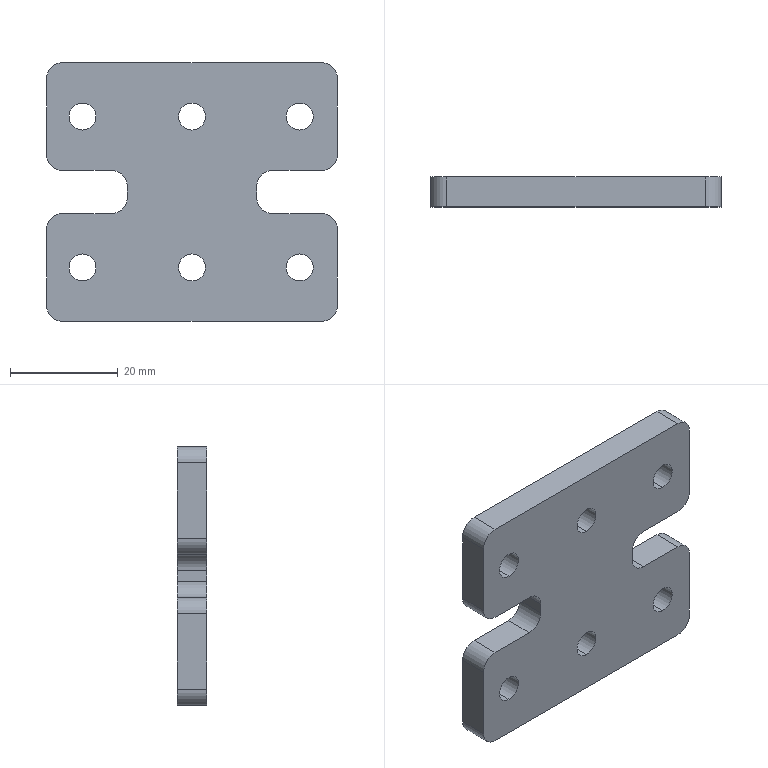Part | SolidWorks | features BaseBody 1 | 1 solid | 38 faces | box 54 x 5.5 x 48 mm | volume 12246 mm3 | cylinder 24 | plane 14 | commonest cylinder face diameters 5 x12 6 x12
STEP:
#1=CARTESIAN_POINT('',(20.,0.,11.5));
#2=VERTEX_POINT('',#1);
#3=CARTESIAN_POINT('',(20.,0.,16.5));
#4=VERTEX_POINT('',#3);
#5=CARTESIAN_POINT('',(20.,0.,14.));
#6=DIRECTION('',(0.,1.,0.));
#7=DIRECTION('',(0.,0.,1.));
#8=AXIS2_PLACEMENT_3D('',#5,#6,#7);
#9=CIRCLE('',#8,2.5);
#10=EDGE_CURVE('',#2,#4,#9,.T.);
#11=ORIENTED_EDGE('',*,*,#10,.F.);
#12=CARTESIAN_POINT('',(20.,5.5,11.5));
#13=VERTEX_POINT('',#12);
#14=CARTESIAN_POINT('',(20.,0.,11.5));
#15=DIRECTION('',(0.,1.,0.));
#16=VECTOR('',#15,1000.);
#17=LINE('',#14,#16);
#18=EDGE_CURVE('',#2,#13,#17,.T.);
#19=ORIENTED_EDGE('',*,*,#18,.T.);
#20=CARTESIAN_POINT('',(20.,5.5,16.5));
#21=VERTEX_POINT('',#20);
#22=CARTESIAN_POINT('',(20.,5.5,14.));
#23=DIRECTION('',(0.,-1.,0.));
#24=DIRECTION('',(0.,0.,1.));
#25=AXIS2_PLACEMENT_3D('',#22,#23,#24);
#26=CIRCLE('',#25,2.5);
#27=EDGE_CURVE('',#21,#13,#26,.T.);
#28=ORIENTED_EDGE('',*,*,#27,.F.);
#29=CARTESIAN_POINT('',(20.,0.,16.5));
#30=DIRECTION('',(0.,1.,0.));
#31=VECTOR('',#30,1000.);
#32=LINE('',#29,#31);
#33=EDGE_CURVE('',#4,#21,#32,.T.);
#34=ORIENTED_EDGE('',*,*,#33,.F.);
#35=EDGE_LOOP('',(#11,#19,#28,#34));
#36=FACE_OUTER_BOUND('',#35,.T.);
#37=CARTESIAN_POINT('',(20.,0.,14.));
#38=DIRECTION('',(0.,1.,0.));
#39=DIRECTION('',(0.,0.,1.));
#40=AXIS2_PLACEMENT_3D('',#37,#38,#39);
#41=CYLINDRICAL_SURFACE('',#40,2.5);
#42=ADVANCED_FACE('',(#36),#41,.F.);
#43=CARTESIAN_POINT('',(0.,0.,-16.5));
#44=VERTEX_POINT('',#43);
#45=CARTESIAN_POINT('',(0.,0.,-11.5));
#46=VERTEX_POINT('',#45);
#47=CARTESIAN_POINT('',(0.,0.,-14.));
#48=DIRECTION('',(0.,1.,0.));
#49=DIRECTION('',(0.,0.,1.));
#50=AXIS2_PLACEMENT_3D('',#47,#48,#49);
#51=CIRCLE('',#50,2.5);
#52=EDGE_CURVE('',#44,#46,#51,.T.);
#53=ORIENTED_EDGE('',*,*,#52,.F.);
#54=CARTESIAN_POINT('',(0.,5.5,-16.5));
#55=VERTEX_POINT('',#54);
#56=CARTESIAN_POINT('',(0.,0.,-16.5));
#57=DIRECTION('',(0.,1.,0.));
#58=VECTOR('',#57,1000.);
#59=LINE('',#56,#58);
#60=EDGE_CURVE('',#44,#55,#59,.T.);
#61=ORIENTED_EDGE('',*,*,#60,.T.);
#62=CARTESIAN_POINT('',(0.,5.5,-11.5));
#63=VERTEX_POINT('',#62);
#64=CARTESIAN_POINT('',(0.,5.5,-14.));
#65=DIRECTION('',(0.,-1.,0.));
#66=DIRECTION('',(0.,0.,1.));
#67=AXIS2_PLACEMENT_3D('',#64,#65,#66);
#68=CIRCLE('',#67,2.5);
#69=EDGE_CURVE('',#63,#55,#68,.T.);
#70=ORIENTED_EDGE('',*,*,#69,.F.);
#71=CARTESIAN_POINT('',(0.,0.,-11.5));
#72=DIRECTION('',(0.,1.,0.));
#73=VECTOR('',#72,1000.);
#74=LINE('',#71,#73);
#75=EDGE_CURVE('',#46,#63,#74,.T.);
#76=ORIENTED_EDGE('',*,*,#75,.F.);
#77=EDGE_LOOP('',(#53,#61,#70,#76));
#78=FACE_OUTER_BOUND('',#77,.T.);
#79=CARTESIAN_POINT('',(0.,0.,-14.));
#80=DIRECTION('',(0.,1.,0.));
#81=DIRECTION('',(0.,0.,1.));
#82=AXIS2_PLACEMENT_3D('',#79,#80,#81);
#83=CYLINDRICAL_SURFACE('',#82,2.5);
#84=ADVANCED_FACE('',(#78),#83,.F.);
#85=CARTESIAN_POINT('',(-20.32,0.,-16.5));
#86=VERTEX_POINT('',#85);
#87=CARTESIAN_POINT('',(-20.32,0.,-11.5));
#88=VERTEX_POINT('',#87);
#89=CARTESIAN_POINT('',(-20.32,0.,-14.));
#90=DIRECTION('',(0.,1.,0.));
#91=DIRECTION('',(0.,0.,1.));
#92=AXIS2_PLACEMENT_3D('',#89,#90,#91);
#93=CIRCLE('',#92,2.5);
#94=EDGE_CURVE('',#86,#88,#93,.T.);
#95=ORIENTED_EDGE('',*,*,#94,.F.);
#96=CARTESIAN_POINT('',(-20.32,5.5,-16.5));
#97=VERTEX_POINT('',#96);
#98=CARTESIAN_POINT('',(-20.32,0.,-16.5));
#99=DIRECTION('',(0.,1.,0.));
#100=VECTOR('',#99,1000.);
#101=LINE('',#98,#100);
#102=EDGE_CURVE('',#86,#97,#101,.T.);
#103=ORIENTED_EDGE('',*,*,#102,.T.);
#104=CARTESIAN_POINT('',(-20.32,5.5,-11.5));
#105=VERTEX_POINT('',#104);
#106=CARTESIAN_POINT('',(-20.32,5.5,-14.));
#107=DIRECTION('',(0.,-1.,0.));
#108=DIRECTION('',(0.,0.,1.));
#109=AXIS2_PLACEMENT_3D('',#106,#107,#108);
#110=CIRCLE('',#109,2.5);
#111=EDGE_CURVE('',#105,#97,#110,.T.);
#112=ORIENTED_EDGE('',*,*,#111,.F.);
#113=CARTESIAN_POINT('',(-20.32,0.,-11.5));
#114=DIRECTION('',(0.,1.,0.));
#115=VECTOR('',#114,1000.);
#116=LINE('',#113,#115);
#117=EDGE_CURVE('',#88,#105,#116,.T.);
#118=ORIENTED_EDGE('',*,*,#117,.F.);
#119=EDGE_LOOP('',(#95,#103,#112,#118));
#120=FACE_OUTER_BOUND('',#119,.T.);
#121=CARTESIAN_POINT('',(-20.32,0.,-14.));
#122=DIRECTION('',(0.,1.,0.));
#123=DIRECTION('',(0.,0.,1.));
#124=AXIS2_PLACEMENT_3D('',#121,#122,#123);
#125=CYLINDRICAL_SURFACE('',#124,2.5);
#126=ADVANCED_FACE('',(#120),#125,.F.);
#127=CARTESIAN_POINT('',(0.,0.,11.5));
#128=VERTEX_POINT('',#127);
#129=CARTESIAN_POINT('',(0.,0.,16.5));
#130=VERTEX_POINT('',#129);
#131=CARTESIAN_POINT('',(0.,0.,14.));
#132=DIRECTION('',(0.,1.,0.));
#133=DIRECTION('',(0.,0.,1.));
#134=AXIS2_PLACEMENT_3D('',#131,#132,#133);
#135=CIRCLE('',#134,2.5);
#136=EDGE_CURVE('',#128,#130,#135,.T.);
#137=ORIENTED_EDGE('',*,*,#136,.F.);
#138=CARTESIAN_POINT('',(0.,5.5,11.5));
#139=VERTEX_POINT('',#138);
#140=CARTESIAN_POINT('',(0.,0.,11.5));
#141=DIRECTION('',(0.,1.,0.));
#142=VECTOR('',#141,1000.);
#143=LINE('',#140,#142);
#144=EDGE_CURVE('',#128,#139,#143,.T.);
#145=ORIENTED_EDGE('',*,*,#144,.T.);
#146=CARTESIAN_POINT('',(0.,5.5,16.5));
#147=VERTEX_POINT('',#146);
#148=CARTESIAN_POINT('',(0.,5.5,14.));
#149=DIRECTION('',(0.,-1.,0.));
#150=DIRECTION('',(0.,0.,1.));
#151=AXIS2_PLACEMENT_3D('',#148,#149,#150);
#152=CIRCLE('',#151,2.5);
#153=EDGE_CURVE('',#147,#139,#152,.T.);
#154=ORIENTED_EDGE('',*,*,#153,.F.);
#155=CARTESIAN_POINT('',(0.,0.,16.5));
#156=DIRECTION('',(0.,1.,0.));
#157=VECTOR('',#156,1000.);
#158=LINE('',#155,#157);
#159=EDGE_CURVE('',#130,#147,#158,.T.);
#160=ORIENTED_EDGE('',*,*,#159,.F.);
#161=EDGE_LOOP('',(#137,#145,#154,#160));
#162=FACE_OUTER_BOUND('',#161,.T.);
#163=CARTESIAN_POINT('',(0.,0.,14.));
#164=DIRECTION('',(0.,1.,0.));
#165=DIRECTION('',(0.,0.,1.));
#166=AXIS2_PLACEMENT_3D('',#163,#164,#165);
#167=CYLINDRICAL_SURFACE('',#166,2.5);
#168=ADVANCED_FACE('',(#162),#167,.F.);
#169=CARTESIAN_POINT('',(-20.32,0.,11.5));
#170=VERTEX_POINT('',#169);
#171=CARTESIAN_POINT('',(-20.32,0.,16.5));
#172=VERTEX_POINT('',#171);
#173=CARTESIAN_POINT('',(-20.32,0.,14.));
#174=DIRECTION('',(0.,1.,0.));
#175=DIRECTION('',(0.,0.,1.));
#176=AXIS2_PLACEMENT_3D('',#173,#174,#175);
#177=CIRCLE('',#176,2.5);
#178=EDGE_CURVE('',#170,#172,#177,.T.);
#179=ORIENTED_EDGE('',*,*,#178,.F.);
#180=CARTESIAN_POINT('',(-20.32,5.5,11.5));
#181=VERTEX_POINT('',#180);
#182=CARTESIAN_POINT('',(-20.32,0.,11.5));
#183=DIRECTION('',(0.,1.,0.));
#184=VECTOR('',#183,1000.);
#185=LINE('',#182,#184);
#186=EDGE_CURVE('',#170,#181,#185,.T.);
#187=ORIENTED_EDGE('',*,*,#186,.T.);
#188=CARTESIAN_POINT('',(-20.32,5.5,16.5));
#189=VERTEX_POINT('',#188);
#190=CARTESIAN_POINT('',(-20.32,5.5,14.));
#191=DIRECTION('',(0.,-1.,0.));
#192=DIRECTION('',(0.,0.,1.));
#193=AXIS2_PLACEMENT_3D('',#190,#191,#192);
#194=CIRCLE('',#193,2.5);
#195=EDGE_CURVE('',#189,#181,#194,.T.);
#196=ORIENTED_EDGE('',*,*,#195,.F.);
#197=CARTESIAN_POINT('',(-20.32,0.,16.5));
#198=DIRECTION('',(0.,1.,0.));
#199=VECTOR('',#198,1000.);
#200=LINE('',#197,#199);
#201=EDGE_CURVE('',#172,#189,#200,.T.);
#202=ORIENTED_EDGE('',*,*,#201,.F.);
#203=EDGE_LOOP('',(#179,#187,#196,#202));
#204=FACE_OUTER_BOUND('',#203,.T.);
#205=CARTESIAN_POINT('',(-20.32,0.,14.));
#206=DIRECTION('',(0.,1.,0.));
#207=DIRECTION('',(0.,0.,1.));
#208=AXIS2_PLACEMENT_3D('',#205,#206,#207);
#209=CYLINDRICAL_SURFACE('',#208,2.5);
#210=ADVANCED_FACE('',(#204),#209,.F.);
#211=CARTESIAN_POINT('',(20.,0.,-16.5));
#212=VERTEX_POINT('',#211);
#213=CARTESIAN_POINT('',(20.,0.,-11.5));
#214=VERTEX_POINT('',#213);
#215=CARTESIAN_POINT('',(20.,0.,-14.));
#216=DIRECTION('',(0.,1.,0.));
#217=DIRECTION('',(0.,0.,1.));
#218=AXIS2_PLACEMENT_3D('',#215,#216,#217);
#219=CIRCLE('',#218,2.5);
#220=EDGE_CURVE('',#212,#214,#219,.T.);
#221=ORIENTED_EDGE('',*,*,#220,.F.);
#222=CARTESIAN_POINT('',(20.,5.5,-16.5));
#223=VERTEX_POINT('',#222);
#224=CARTESIAN_POINT('',(20.,0.,-16.5));
#225=DIRECTION('',(0.,1.,0.));
#226=VECTOR('',#225,1000.);
#227=LINE('',#224,#226);
#228=EDGE_CURVE('',#212,#223,#227,.T.);
#229=ORIENTED_EDGE('',*,*,#228,.T.);
#230=CARTESIAN_POINT('',(20.,5.5,-11.5));
#231=VERTEX_POINT('',#230);
#232=CARTESIAN_POINT('',(20.,5.5,-14.));
#233=DIRECTION('',(0.,-1.,0.));
#234=DIRECTION('',(0.,0.,1.));
#235=AXIS2_PLACEMENT_3D('',#232,#233,#234);
#236=CIRCLE('',#235,2.5);
#237=EDGE_CURVE('',#231,#223,#236,.T.);
#238=ORIENTED_EDGE('',*,*,#237,.F.);
#239=CARTESIAN_POINT('',(20.,0.,-11.5));
#240=DIRECTION('',(0.,1.,0.));
#241=VECTOR('',#240,1000.);
#242=LINE('',#239,#241);
#243=EDGE_CURVE('',#214,#231,#242,.T.);
#244=ORIENTED_EDGE('',*,*,#243,.F.);
#245=EDGE_LOOP('',(#221,#229,#238,#244));
#246=FACE_OUTER_BOUND('',#245,.T.);
#247=CARTESIAN_POINT('',(20.,0.,-14.));
#248=DIRECTION('',(0.,1.,0.));
#249=DIRECTION('',(0.,0.,1.));
#250=AXIS2_PLACEMENT_3D('',#247,#248,#249);
#251=CYLINDRICAL_SURFACE('',#250,2.5);
#252=ADVANCED_FACE('',(#246),#251,.F.);
#253=CARTESIAN_POINT('',(20.,0.,14.));
#254=DIRECTION('',(0.,1.,0.));
#255=DIRECTION('',(0.,0.,1.));
#256=AXIS2_PLACEMENT_3D('',#253,#254,#255);
#257=CIRCLE('',#256,2.5);
#258=EDGE_CURVE('',#4,#2,#257,.T.);
#259=ORIENTED_EDGE('',*,*,#258,.T.);
#260=ORIENTED_EDGE('',*,*,#10,.T.);
#261=EDGE_LOOP('',(#259,#260));
#262=FACE_BOUND('',#261,.T.);
#263=CARTESIAN_POINT('',(0.,0.,-14.));
#264=DIRECTION('',(0.,1.,0.));
#265=DIRECTION('',(0.,0.,1.));
#266=AXIS2_PLACEMENT_3D('',#263,#264,#265);
#267=CIRCLE('',#266,2.5);
#268=EDGE_CURVE('',#46,#44,#267,.T.);
#269=ORIENTED_EDGE('',*,*,#268,.T.);
#270=ORIENTED_EDGE('',*,*,#52,.T.);
#271=EDGE_LOOP('',(#269,#270));
#272=FACE_BOUND('',#271,.T.);
#273=CARTESIAN_POINT('',(-20.32,0.,-14.));
#274=DIRECTION('',(0.,1.,0.));
#275=DIRECTION('',(0.,0.,1.));
#276=AXIS2_PLACEMENT_3D('',#273,#274,#275);
#277=CIRCLE('',#276,2.5);
#278=EDGE_CURVE('',#88,#86,#277,.T.);
#279=ORIENTED_EDGE('',*,*,#278,.T.);
#280=ORIENTED_EDGE('',*,*,#94,.T.);
#281=EDGE_LOOP('',(#279,#280));
#282=FACE_BOUND('',#281,.T.);
#283=CARTESIAN_POINT('',(0.,0.,14.));
#284=DIRECTION('',(0.,1.,0.));
#285=DIRECTION('',(0.,0.,1.));
#286=AXIS2_PLACEMENT_3D('',#283,#284,#285);
#287=CIRCLE('',#286,2.5);
#288=EDGE_CURVE('',#130,#128,#287,.T.);
#289=ORIENTED_EDGE('',*,*,#288,.T.);
#290=ORIENTED_EDGE('',*,*,#136,.T.);
#291=EDGE_LOOP('',(#289,#290));
#292=FACE_BOUND('',#291,.T.);
#293=CARTESIAN_POINT('',(-20.32,0.,14.));
#294=DIRECTION('',(0.,1.,0.));
#295=DIRECTION('',(0.,0.,1.));
#296=AXIS2_PLACEMENT_3D('',#293,#294,#295);
#297=CIRCLE('',#296,2.5);
#298=EDGE_CURVE('',#172,#170,#297,.T.);
#299=ORIENTED_EDGE('',*,*,#298,.T.);
#300=ORIENTED_EDGE('',*,*,#178,.T.);
#301=EDGE_LOOP('',(#299,#300));
#302=FACE_BOUND('',#301,.T.);
#303=CARTESIAN_POINT('',(20.,0.,-14.));
#304=DIRECTION('',(0.,1.,0.));
#305=DIRECTION('',(0.,0.,1.));
#306=AXIS2_PLACEMENT_3D('',#303,#304,#305);
#307=CIRCLE('',#306,2.5);
#308=EDGE_CURVE('',#214,#212,#307,.T.);
#309=ORIENTED_EDGE('',*,*,#308,.T.);
#310=ORIENTED_EDGE('',*,*,#220,.T.);
#311=EDGE_LOOP('',(#309,#310));
#312=FACE_BOUND('',#311,.T.);
#313=CARTESIAN_POINT('',(12.,0.,-1.));
#314=VERTEX_POINT('',#313);
#315=CARTESIAN_POINT('',(12.,0.,1.));
#316=VERTEX_POINT('',#315);
#317=CARTESIAN_POINT('',(12.,0.,0.));
#318=DIRECTION('',(0.,0.,1.));
#319=VECTOR('',#318,1000.);
#320=LINE('',#317,#319);
#321=EDGE_CURVE('',#314,#316,#320,.T.);
#322=ORIENTED_EDGE('',*,*,#321,.T.);
#323=CARTESIAN_POINT('',(15.,0.,4.));
#324=VERTEX_POINT('',#323);
#325=CARTESIAN_POINT('',(15.,0.,1.));
#326=DIRECTION('',(0.,1.,0.));
#327=DIRECTION('',(0.,0.,-1.));
#328=AXIS2_PLACEMENT_3D('',#325,#326,#327);
#329=CIRCLE('',#328,3.);
#330=EDGE_CURVE('',#316,#324,#329,.T.);
#331=ORIENTED_EDGE('',*,*,#330,.T.);
#332=CARTESIAN_POINT('',(24.,0.,4.));
#333=VERTEX_POINT('',#332);
#334=CARTESIAN_POINT('',(0.,0.,4.));
#335=DIRECTION('',(1.,0.,0.));
#336=VECTOR('',#335,1000.);
#337=LINE('',#334,#336);
#338=EDGE_CURVE('',#324,#333,#337,.T.);
#339=ORIENTED_EDGE('',*,*,#338,.T.);
#340=CARTESIAN_POINT('',(27.,0.,7.));
#341=VERTEX_POINT('',#340);
#342=CARTESIAN_POINT('',(24.,0.,7.));
#343=DIRECTION('',(0.,-1.,0.));
#344=DIRECTION('',(0.,0.,-1.));
#345=AXIS2_PLACEMENT_3D('',#342,#343,#344);
#346=CIRCLE('',#345,3.);
#347=EDGE_CURVE('',#333,#341,#346,.T.);
#348=ORIENTED_EDGE('',*,*,#347,.T.);
#349=CARTESIAN_POINT('',(27.,0.,21.));
#350=VERTEX_POINT('',#349);
#351=CARTESIAN_POINT('',(27.,0.,0.));
#352=DIRECTION('',(0.,0.,1.));
#353=VECTOR('',#352,1000.);
#354=LINE('',#351,#353);
#355=EDGE_CURVE('',#341,#350,#354,.T.);
#356=ORIENTED_EDGE('',*,*,#355,.T.);
#357=CARTESIAN_POINT('',(24.,0.,24.));
#358=VERTEX_POINT('',#357);
#359=CARTESIAN_POINT('',(24.,0.,21.));
#360=DIRECTION('',(0.,-1.,0.));
#361=DIRECTION('',(0.,0.,-1.));
#362=AXIS2_PLACEMENT_3D('',#359,#360,#361);
#363=CIRCLE('',#362,3.);
#364=EDGE_CURVE('',#350,#358,#363,.T.);
#365=ORIENTED_EDGE('',*,*,#364,.T.);
#366=CARTESIAN_POINT('',(-24.,0.,24.));
#367=VERTEX_POINT('',#366);
#368=CARTESIAN_POINT('',(0.,0.,24.));
#369=DIRECTION('',(-1.,0.,0.));
#370=VECTOR('',#369,1000.);
#371=LINE('',#368,#370);
#372=EDGE_CURVE('',#358,#367,#371,.T.);
#373=ORIENTED_EDGE('',*,*,#372,.T.);
#374=CARTESIAN_POINT('',(-27.,0.,21.));
#375=VERTEX_POINT('',#374);
#376=CARTESIAN_POINT('',(-24.,0.,21.));
#377=DIRECTION('',(0.,-1.,0.));
#378=DIRECTION('',(0.,0.,-1.));
#379=AXIS2_PLACEMENT_3D('',#376,#377,#378);
#380=CIRCLE('',#379,3.);
#381=EDGE_CURVE('',#367,#375,#380,.T.);
#382=ORIENTED_EDGE('',*,*,#381,.T.);
#383=CARTESIAN_POINT('',(-27.,0.,7.));
#384=VERTEX_POINT('',#383);
#385=CARTESIAN_POINT('',(-27.,0.,0.));
#386=DIRECTION('',(0.,0.,-1.));
#387=VECTOR('',#386,1000.);
#388=LINE('',#385,#387);
#389=EDGE_CURVE('',#375,#384,#388,.T.);
#390=ORIENTED_EDGE('',*,*,#389,.T.);
#391=CARTESIAN_POINT('',(-24.,0.,4.));
#392=VERTEX_POINT('',#391);
#393=CARTESIAN_POINT('',(-24.,0.,7.));
#394=DIRECTION('',(0.,-1.,0.));
#395=DIRECTION('',(0.,0.,1.));
#396=AXIS2_PLACEMENT_3D('',#393,#394,#395);
#397=CIRCLE('',#396,3.);
#398=EDGE_CURVE('',#384,#392,#397,.T.);
#399=ORIENTED_EDGE('',*,*,#398,.T.);
#400=CARTESIAN_POINT('',(-15.,0.,4.));
#401=VERTEX_POINT('',#400);
#402=CARTESIAN_POINT('',(0.,0.,4.));
#403=DIRECTION('',(1.,0.,0.));
#404=VECTOR('',#403,1000.);
#405=LINE('',#402,#404);
#406=EDGE_CURVE('',#392,#401,#405,.T.);
#407=ORIENTED_EDGE('',*,*,#406,.T.);
#408=CARTESIAN_POINT('',(-12.,0.,1.));
#409=VERTEX_POINT('',#408);
#410=CARTESIAN_POINT('',(-15.,0.,1.));
#411=DIRECTION('',(0.,1.,0.));
#412=DIRECTION('',(0.,0.,-1.));
#413=AXIS2_PLACEMENT_3D('',#410,#411,#412);
#414=CIRCLE('',#413,3.);
#415=EDGE_CURVE('',#401,#409,#414,.T.);
#416=ORIENTED_EDGE('',*,*,#415,.T.);
#417=CARTESIAN_POINT('',(-12.,0.,-1.));
#418=VERTEX_POINT('',#417);
#419=CARTESIAN_POINT('',(-12.,0.,0.));
#420=DIRECTION('',(0.,0.,-1.));
#421=VECTOR('',#420,1000.);
#422=LINE('',#419,#421);
#423=EDGE_CURVE('',#409,#418,#422,.T.);
#424=ORIENTED_EDGE('',*,*,#423,.T.);
#425=CARTESIAN_POINT('',(-15.,0.,-4.));
#426=VERTEX_POINT('',#425);
#427=CARTESIAN_POINT('',(-15.,0.,-1.));
#428=DIRECTION('',(0.,1.,0.));
#429=DIRECTION('',(0.,0.,-1.));
#430=AXIS2_PLACEMENT_3D('',#427,#428,#429);
#431=CIRCLE('',#430,3.);
#432=EDGE_CURVE('',#418,#426,#431,.T.);
#433=ORIENTED_EDGE('',*,*,#432,.T.);
#434=CARTESIAN_POINT('',(-24.,0.,-4.));
#435=VERTEX_POINT('',#434);
#436=CARTESIAN_POINT('',(0.,0.,-4.));
#437=DIRECTION('',(-1.,0.,0.));
#438=VECTOR('',#437,1000.);
#439=LINE('',#436,#438);
#440=EDGE_CURVE('',#426,#435,#439,.T.);
#441=ORIENTED_EDGE('',*,*,#440,.T.);
#442=CARTESIAN_POINT('',(-27.,0.,-7.));
#443=VERTEX_POINT('',#442);
#444=CARTESIAN_POINT('',(-24.,0.,-7.));
#445=DIRECTION('',(0.,-1.,0.));
#446=DIRECTION('',(0.,0.,-1.));
#447=AXIS2_PLACEMENT_3D('',#444,#445,#446);
#448=CIRCLE('',#447,3.);
#449=EDGE_CURVE('',#435,#443,#448,.T.);
#450=ORIENTED_EDGE('',*,*,#449,.T.);
#451=CARTESIAN_POINT('',(-27.,0.,-21.));
#452=VERTEX_POINT('',#451);
#453=CARTESIAN_POINT('',(-27.,0.,0.));
#454=DIRECTION('',(0.,0.,-1.));
#455=VECTOR('',#454,1000.);
#456=LINE('',#453,#455);
#457=EDGE_CURVE('',#443,#452,#456,.T.);
#458=ORIENTED_EDGE('',*,*,#457,.T.);
#459=CARTESIAN_POINT('',(-24.,0.,-24.));
#460=VERTEX_POINT('',#459);
#461=CARTESIAN_POINT('',(-24.,0.,-21.));
#462=DIRECTION('',(0.,-1.,0.));
#463=DIRECTION('',(0.,0.,-1.));
#464=AXIS2_PLACEMENT_3D('',#461,#462,#463);
#465=CIRCLE('',#464,3.);
#466=EDGE_CURVE('',#452,#460,#465,.T.);
#467=ORIENTED_EDGE('',*,*,#466,.T.);
#468=CARTESIAN_POINT('',(24.,0.,-24.));
#469=VERTEX_POINT('',#468);
#470=CARTESIAN_POINT('',(0.,0.,-24.));
#471=DIRECTION('',(1.,0.,0.));
#472=VECTOR('',#471,1000.);
#473=LINE('',#470,#472);
#474=EDGE_CURVE('',#460,#469,#473,.T.);
#475=ORIENTED_EDGE('',*,*,#474,.T.);
#476=CARTESIAN_POINT('',(27.,0.,-21.));
#477=VERTEX_POINT('',#476);
#478=CARTESIAN_POINT('',(24.,0.,-21.));
#479=DIRECTION('',(0.,-1.,0.));
#480=DIRECTION('',(0.,0.,-1.));
#481=AXIS2_PLACEMENT_3D('',#478,#479,#480);
#482=CIRCLE('',#481,3.);
#483=EDGE_CURVE('',#469,#477,#482,.T.);
#484=ORIENTED_EDGE('',*,*,#483,.T.);
#485=CARTESIAN_POINT('',(27.,0.,-7.));
#486=VERTEX_POINT('',#485);
#487=CARTESIAN_POINT('',(27.,0.,0.));
#488=DIRECTION('',(0.,0.,1.));
#489=VECTOR('',#488,1000.);
#490=LINE('',#487,#489);
#491=EDGE_CURVE('',#477,#486,#490,.T.);
#492=ORIENTED_EDGE('',*,*,#491,.T.);
#493=CARTESIAN_POINT('',(24.,0.,-4.));
#494=VERTEX_POINT('',#493);
#495=CARTESIAN_POINT('',(24.,0.,-7.));
#496=DIRECTION('',(0.,-1.,0.));
#497=DIRECTION('',(0.,0.,1.));
#498=AXIS2_PLACEMENT_3D('',#495,#496,#497);
#499=CIRCLE('',#498,3.);
#500=EDGE_CURVE('',#486,#494,#499,.T.);
#501=ORIENTED_EDGE('',*,*,#500,.T.);
#502=CARTESIAN_POINT('',(15.,0.,-4.));
#503=VERTEX_POINT('',#502);
#504=CARTESIAN_POINT('',(0.,0.,-4.));
#505=DIRECTION('',(-1.,0.,0.));
#506=VECTOR('',#505,1000.);
#507=LINE('',#504,#506);
#508=EDGE_CURVE('',#494,#503,#507,.T.);
#509=ORIENTED_EDGE('',*,*,#508,.T.);
#510=CARTESIAN_POINT('',(15.,0.,-1.));
#511=DIRECTION('',(0.,1.,0.));
#512=DIRECTION('',(0.,0.,-1.));
#513=AXIS2_PLACEMENT_3D('',#510,#511,#512);
#514=CIRCLE('',#513,3.);
#515=EDGE_CURVE('',#503,#314,#514,.T.);
#516=ORIENTED_EDGE('',*,*,#515,.T.);
#517=EDGE_LOOP('',(#322,#331,#339,#348,#356,#365,#373,#382,#390,#399,#407,#416,#424,#433,#441,#450,#458,#467,#475,#484,#492,#501,#509,#516));
#518=FACE_OUTER_BOUND('',#517,.T.);
#519=CARTESIAN_POINT('',(0.,0.,0.));
#520=DIRECTION('',(0.,-1.,0.));
#521=DIRECTION('',(0.,0.,-1.));
#522=AXIS2_PLACEMENT_3D('',#519,#520,#521);
#523=PLANE('',#522);
#524=ADVANCED_FACE('',(#262,#272,#282,#292,#302,#312,#518),#523,.T.);
#525=ORIENTED_EDGE('',*,*,#18,.F.);
#526=ORIENTED_EDGE('',*,*,#258,.F.);
#527=ORIENTED_EDGE('',*,*,#33,.T.);
#528=CARTESIAN_POINT('',(20.,5.5,14.));
#529=DIRECTION('',(0.,-1.,0.));
#530=DIRECTION('',(0.,0.,1.));
#531=AXIS2_PLACEMENT_3D('',#528,#529,#530);
#532=CIRCLE('',#531,2.5);
#533=EDGE_CURVE('',#13,#21,#532,.T.);
#534=ORIENTED_EDGE('',*,*,#533,.F.);
#535=EDGE_LOOP('',(#525,#526,#527,#534));
#536=FACE_OUTER_BOUND('',#535,.T.);
#537=CARTESIAN_POINT('',(20.,0.,14.));
#538=DIRECTION('',(0.,1.,0.));
#539=DIRECTION('',(0.,0.,1.));
#540=AXIS2_PLACEMENT_3D('',#537,#538,#539);
#541=CYLINDRICAL_SURFACE('',#540,2.5);
#542=ADVANCED_FACE('',(#536),#541,.F.);
#543=ORIENTED_EDGE('',*,*,#60,.F.);
#544=ORIENTED_EDGE('',*,*,#268,.F.);
#545=ORIENTED_EDGE('',*,*,#75,.T.);
#546=CARTESIAN_POINT('',(0.,5.5,-14.));
#547=DIRECTION('',(0.,-1.,0.));
#548=DIRECTION('',(0.,0.,1.));
#549=AXIS2_PLACEMENT_3D('',#546,#547,#548);
#550=CIRCLE('',#549,2.5);
#551=EDGE_CURVE('',#55,#63,#550,.T.);
#552=ORIENTED_EDGE('',*,*,#551,.F.);
#553=EDGE_LOOP('',(#543,#544,#545,#552));
#554=FACE_OUTER_BOUND('',#553,.T.);
#555=CARTESIAN_POINT('',(0.,0.,-14.));
#556=DIRECTION('',(0.,1.,0.));
#557=DIRECTION('',(0.,0.,1.));
#558=AXIS2_PLACEMENT_3D('',#555,#556,#557);
#559=CYLINDRICAL_SURFACE('',#558,2.5);
#560=ADVANCED_FACE('',(#554),#559,.F.);
#561=ORIENTED_EDGE('',*,*,#102,.F.);
#562=ORIENTED_EDGE('',*,*,#278,.F.);
#563=ORIENTED_EDGE('',*,*,#117,.T.);
#564=CARTESIAN_POINT('',(-20.32,5.5,-14.));
#565=DIRECTION('',(0.,-1.,0.));
#566=DIRECTION('',(0.,0.,1.));
#567=AXIS2_PLACEMENT_3D('',#564,#565,#566);
#568=CIRCLE('',#567,2.5);
#569=EDGE_CURVE('',#97,#105,#568,.T.);
#570=ORIENTED_EDGE('',*,*,#569,.F.);
#571=EDGE_LOOP('',(#561,#562,#563,#570));
#572=FACE_OUTER_BOUND('',#571,.T.);
#573=CARTESIAN_POINT('',(-20.32,0.,-14.));
#574=DIRECTION('',(0.,1.,0.));
#575=DIRECTION('',(0.,0.,1.));
#576=AXIS2_PLACEMENT_3D('',#573,#574,#575);
#577=CYLINDRICAL_SURFACE('',#576,2.5);
#578=ADVANCED_FACE('',(#572),#577,.F.);
#579=ORIENTED_EDGE('',*,*,#144,.F.);
#580=ORIENTED_EDGE('',*,*,#288,.F.);
#581=ORIENTED_EDGE('',*,*,#159,.T.);
#582=CARTESIAN_POINT('',(0.,5.5,14.));
#583=DIRECTION('',(0.,-1.,0.));
#584=DIRECTION('',(0.,0.,1.));
#585=AXIS2_PLACEMENT_3D('',#582,#583,#584);
#586=CIRCLE('',#585,2.5);
#587=EDGE_CURVE('',#139,#147,#586,.T.);
#588=ORIENTED_EDGE('',*,*,#587,.F.);
#589=EDGE_LOOP('',(#579,#580,#581,#588));
#590=FACE_OUTER_BOUND('',#589,.T.);
#591=CARTESIAN_POINT('',(0.,0.,14.));
#592=DIRECTION('',(0.,1.,0.));
#593=DIRECTION('',(0.,0.,1.));
#594=AXIS2_PLACEMENT_3D('',#591,#592,#593);
#595=CYLINDRICAL_SURFACE('',#594,2.5);
#596=ADVANCED_FACE('',(#590),#595,.F.);
#597=ORIENTED_EDGE('',*,*,#186,.F.);
#598=ORIENTED_EDGE('',*,*,#298,.F.);
#599=ORIENTED_EDGE('',*,*,#201,.T.);
#600=CARTESIAN_POINT('',(-20.32,5.5,14.));
#601=DIRECTION('',(0.,-1.,0.));
#602=DIRECTION('',(0.,0.,1.));
#603=AXIS2_PLACEMENT_3D('',#600,#601,#602);
#604=CIRCLE('',#603,2.5);
#605=EDGE_CURVE('',#181,#189,#604,.T.);
#606=ORIENTED_EDGE('',*,*,#605,.F.);
#607=EDGE_LOOP('',(#597,#598,#599,#606));
#608=FACE_OUTER_BOUND('',#607,.T.);
#609=CARTESIAN_POINT('',(-20.32,0.,14.));
#610=DIRECTION('',(0.,1.,0.));
#611=DIRECTION('',(0.,0.,1.));
#612=AXIS2_PLACEMENT_3D('',#609,#610,#611);
#613=CYLINDRICAL_SURFACE('',#612,2.5);
#614=ADVANCED_FACE('',(#608),#613,.F.);
#615=ORIENTED_EDGE('',*,*,#228,.F.);
#616=ORIENTED_EDGE('',*,*,#308,.F.);
#617=ORIENTED_EDGE('',*,*,#243,.T.);
#618=CARTESIAN_POINT('',(20.,5.5,-14.));
#619=DIRECTION('',(0.,-1.,0.));
#620=DIRECTION('',(0.,0.,1.));
#621=AXIS2_PLACEMENT_3D('',#618,#619,#620);
#622=CIRCLE('',#621,2.5);
#623=EDGE_CURVE('',#223,#231,#622,.T.);
#624=ORIENTED_EDGE('',*,*,#623,.F.);
#625=EDGE_LOOP('',(#615,#616,#617,#624));
#626=FACE_OUTER_BOUND('',#625,.T.);
#627=CARTESIAN_POINT('',(20.,0.,-14.));
#628=DIRECTION('',(0.,1.,0.));
#629=DIRECTION('',(0.,0.,1.));
#630=AXIS2_PLACEMENT_3D('',#627,#628,#629);
#631=CYLINDRICAL_SURFACE('',#630,2.5);
#632=ADVANCED_FACE('',(#626),#631,.F.);
#633=CARTESIAN_POINT('',(12.,5.5,1.));
#634=VERTEX_POINT('',#633);
#635=CARTESIAN_POINT('',(12.,-0.001,1.));
#636=DIRECTION('',(0.,-1.,0.));
#637=VECTOR('',#636,1000.);
#638=LINE('',#635,#637);
#639=EDGE_CURVE('',#634,#316,#638,.T.);
#640=ORIENTED_EDGE('',*,*,#639,.F.);
#641=CARTESIAN_POINT('',(15.,5.5,4.));
#642=VERTEX_POINT('',#641);
#643=CARTESIAN_POINT('',(15.,5.5,1.));
#644=DIRECTION('',(0.,-1.,0.));
#645=DIRECTION('',(0.,0.,-1.));
#646=AXIS2_PLACEMENT_3D('',#643,#644,#645);
#647=CIRCLE('',#646,3.);
#648=EDGE_CURVE('',#642,#634,#647,.T.);
#649=ORIENTED_EDGE('',*,*,#648,.F.);
#650=CARTESIAN_POINT('',(15.,-0.001,4.));
#651=DIRECTION('',(0.,1.,0.));
#652=VECTOR('',#651,1000.);
#653=LINE('',#650,#652);
#654=EDGE_CURVE('',#324,#642,#653,.T.);
#655=ORIENTED_EDGE('',*,*,#654,.F.);
#656=ORIENTED_EDGE('',*,*,#330,.F.);
#657=EDGE_LOOP('',(#640,#649,#655,#656));
#658=FACE_OUTER_BOUND('',#657,.T.);
#659=CARTESIAN_POINT('',(15.,-0.001,1.));
#660=DIRECTION('',(0.,-1.,0.));
#661=DIRECTION('',(0.,0.,-1.));
#662=AXIS2_PLACEMENT_3D('',#659,#660,#661);
#663=CYLINDRICAL_SURFACE('',#662,3.);
#664=ADVANCED_FACE('',(#658),#663,.F.);
#665=ORIENTED_EDGE('',*,*,#639,.T.);
#666=ORIENTED_EDGE('',*,*,#321,.F.);
#667=CARTESIAN_POINT('',(12.,5.5,-1.));
#668=VERTEX_POINT('',#667);
#669=CARTESIAN_POINT('',(12.,-0.001,-1.));
#670=DIRECTION('',(0.,-1.,0.));
#671=VECTOR('',#670,1000.);
#672=LINE('',#669,#671);
#673=EDGE_CURVE('',#668,#314,#672,.T.);
#674=ORIENTED_EDGE('',*,*,#673,.F.);
#675=CARTESIAN_POINT('',(12.,5.5,-4.));
#676=DIRECTION('',(0.,0.,-1.));
#677=VECTOR('',#676,1000.);
#678=LINE('',#675,#677);
#679=EDGE_CURVE('',#634,#668,#678,.T.);
#680=ORIENTED_EDGE('',*,*,#679,.F.);
#681=EDGE_LOOP('',(#665,#666,#674,#680));
#682=FACE_OUTER_BOUND('',#681,.T.);
#683=CARTESIAN_POINT('',(12.,-0.001,-4.));
#684=DIRECTION('',(-1.,0.,0.));
#685=DIRECTION('',(0.,0.,1.));
#686=AXIS2_PLACEMENT_3D('',#683,#684,#685);
#687=PLANE('',#686);
#688=ADVANCED_FACE('',(#682),#687,.F.);
#689=CARTESIAN_POINT('',(15.,5.5,-4.));
#690=VERTEX_POINT('',#689);
#691=CARTESIAN_POINT('',(15.,-0.001,-4.));
#692=DIRECTION('',(0.,-1.,0.));
#693=VECTOR('',#692,1000.);
#694=LINE('',#691,#693);
#695=EDGE_CURVE('',#690,#503,#694,.T.);
#696=ORIENTED_EDGE('',*,*,#695,.F.);
#697=CARTESIAN_POINT('',(15.,5.5,-1.));
#698=DIRECTION('',(0.,-1.,0.));
#699=DIRECTION('',(0.,0.,-1.));
#700=AXIS2_PLACEMENT_3D('',#697,#698,#699);
#701=CIRCLE('',#700,3.);
#702=EDGE_CURVE('',#668,#690,#701,.T.);
#703=ORIENTED_EDGE('',*,*,#702,.F.);
#704=ORIENTED_EDGE('',*,*,#673,.T.);
#705=ORIENTED_EDGE('',*,*,#515,.F.);
#706=EDGE_LOOP('',(#696,#703,#704,#705));
#707=FACE_OUTER_BOUND('',#706,.T.);
#708=CARTESIAN_POINT('',(15.,-0.001,-1.));
#709=DIRECTION('',(0.,-1.,0.));
#710=DIRECTION('',(0.,0.,-1.));
#711=AXIS2_PLACEMENT_3D('',#708,#709,#710);
#712=CYLINDRICAL_SURFACE('',#711,3.);
#713=ADVANCED_FACE('',(#707),#712,.F.);
#714=CARTESIAN_POINT('',(24.,5.5,-4.));
#715=VERTEX_POINT('',#714);
#716=CARTESIAN_POINT('',(24.,-0.001,-4.));
#717=DIRECTION('',(0.,-1.,0.));
#718=VECTOR('',#717,1000.);
#719=LINE('',#716,#718);
#720=EDGE_CURVE('',#715,#494,#719,.T.);
#721=ORIENTED_EDGE('',*,*,#720,.F.);
#722=CARTESIAN_POINT('',(42.,5.5,-4.));
#723=DIRECTION('',(1.,0.,0.));
#724=VECTOR('',#723,1000.);
#725=LINE('',#722,#724);
#726=EDGE_CURVE('',#690,#715,#725,.T.);
#727=ORIENTED_EDGE('',*,*,#726,.F.);
#728=ORIENTED_EDGE('',*,*,#695,.T.);
#729=ORIENTED_EDGE('',*,*,#508,.F.);
#730=EDGE_LOOP('',(#721,#727,#728,#729));
#731=FACE_OUTER_BOUND('',#730,.T.);
#732=CARTESIAN_POINT('',(42.,-0.001,-4.));
#733=DIRECTION('',(0.,0.,-1.));
#734=DIRECTION('',(-1.,0.,0.));
#735=AXIS2_PLACEMENT_3D('',#732,#733,#734);
#736=PLANE('',#735);
#737=ADVANCED_FACE('',(#731),#736,.F.);
#738=CARTESIAN_POINT('',(27.,5.5,-7.));
#739=VERTEX_POINT('',#738);
#740=CARTESIAN_POINT('',(24.,5.5,-7.));
#741=DIRECTION('',(0.,-1.,0.));
#742=DIRECTION('',(0.,0.,1.));
#743=AXIS2_PLACEMENT_3D('',#740,#741,#742);
#744=CIRCLE('',#743,3.);
#745=EDGE_CURVE('',#739,#715,#744,.T.);
#746=ORIENTED_EDGE('',*,*,#745,.T.);
#747=ORIENTED_EDGE('',*,*,#720,.T.);
#748=ORIENTED_EDGE('',*,*,#500,.F.);
#749=CARTESIAN_POINT('',(27.,-0.001,-7.));
#750=DIRECTION('',(0.,1.,0.));
#751=VECTOR('',#750,1000.);
#752=LINE('',#749,#751);
#753=EDGE_CURVE('',#486,#739,#752,.T.);
#754=ORIENTED_EDGE('',*,*,#753,.T.);
#755=EDGE_LOOP('',(#746,#747,#748,#754));
#756=FACE_OUTER_BOUND('',#755,.T.);
#757=CARTESIAN_POINT('',(24.,-0.001,-7.));
#758=DIRECTION('',(0.,1.,0.));
#759=DIRECTION('',(0.,0.,1.));
#760=AXIS2_PLACEMENT_3D('',#757,#758,#759);
#761=CYLINDRICAL_SURFACE('',#760,3.);
#762=ADVANCED_FACE('',(#756),#761,.T.);
#763=ORIENTED_EDGE('',*,*,#753,.F.);
#764=ORIENTED_EDGE('',*,*,#491,.F.);
#765=CARTESIAN_POINT('',(27.,5.5,-21.));
#766=VERTEX_POINT('',#765);
#767=CARTESIAN_POINT('',(27.,5.5,-21.));
#768=DIRECTION('',(0.,-1.,0.));
#769=VECTOR('',#768,1000.);
#770=LINE('',#767,#769);
#771=EDGE_CURVE('',#766,#477,#770,.T.);
#772=ORIENTED_EDGE('',*,*,#771,.F.);
#773=CARTESIAN_POINT('',(27.,5.5,24.));
#774=DIRECTION('',(0.,0.,-1.));
#775=VECTOR('',#774,1000.);
#776=LINE('',#773,#775);
#777=EDGE_CURVE('',#739,#766,#776,.T.);
#778=ORIENTED_EDGE('',*,*,#777,.F.);
#779=EDGE_LOOP('',(#763,#764,#772,#778));
#780=FACE_OUTER_BOUND('',#779,.T.);
#781=CARTESIAN_POINT('',(27.,5.5,24.));
#782=DIRECTION('',(-1.,0.,0.));
#783=DIRECTION('',(0.,0.,1.));
#784=AXIS2_PLACEMENT_3D('',#781,#782,#783);
#785=PLANE('',#784);
#786=ADVANCED_FACE('',(#780),#785,.F.);
#787=ORIENTED_EDGE('',*,*,#483,.F.);
#788=CARTESIAN_POINT('',(24.,5.5,-24.));
#789=VERTEX_POINT('',#788);
#790=CARTESIAN_POINT('',(24.,5.5,-24.));
#791=DIRECTION('',(0.,1.,0.));
#792=VECTOR('',#791,1000.);
#793=LINE('',#790,#792);
#794=EDGE_CURVE('',#469,#789,#793,.T.);
#795=ORIENTED_EDGE('',*,*,#794,.T.);
#796=CARTESIAN_POINT('',(24.,5.5,-21.));
#797=DIRECTION('',(0.,-1.,0.));
#798=DIRECTION('',(0.,0.,-1.));
#799=AXIS2_PLACEMENT_3D('',#796,#797,#798);
#800=CIRCLE('',#799,3.);
#801=EDGE_CURVE('',#789,#766,#800,.T.);
#802=ORIENTED_EDGE('',*,*,#801,.T.);
#803=ORIENTED_EDGE('',*,*,#771,.T.);
#804=EDGE_LOOP('',(#787,#795,#802,#803));
#805=FACE_OUTER_BOUND('',#804,.T.);
#806=CARTESIAN_POINT('',(24.,5.5,-21.));
#807=DIRECTION('',(0.,-1.,0.));
#808=DIRECTION('',(0.,0.,-1.));
#809=AXIS2_PLACEMENT_3D('',#806,#807,#808);
#810=CYLINDRICAL_SURFACE('',#809,3.);
#811=ADVANCED_FACE('',(#805),#810,.T.);
#812=CARTESIAN_POINT('',(-24.,5.5,-24.));
#813=VERTEX_POINT('',#812);
#814=CARTESIAN_POINT('',(-24.,5.5,-24.));
#815=DIRECTION('',(0.,-1.,0.));
#816=VECTOR('',#815,1000.);
#817=LINE('',#814,#816);
#818=EDGE_CURVE('',#813,#460,#817,.T.);
#819=ORIENTED_EDGE('',*,*,#818,.F.);
#820=CARTESIAN_POINT('',(-27.,5.5,-24.));
#821=DIRECTION('',(-1.,0.,0.));
#822=VECTOR('',#821,1000.);
#823=LINE('',#820,#822);
#824=EDGE_CURVE('',#789,#813,#823,.T.);
#825=ORIENTED_EDGE('',*,*,#824,.F.);
#826=ORIENTED_EDGE('',*,*,#794,.F.);
#827=ORIENTED_EDGE('',*,*,#474,.F.);
#828=EDGE_LOOP('',(#819,#825,#826,#827));
#829=FACE_OUTER_BOUND('',#828,.T.);
#830=CARTESIAN_POINT('',(-27.,5.5,-24.));
#831=DIRECTION('',(0.,0.,1.));
#832=DIRECTION('',(1.,0.,0.));
#833=AXIS2_PLACEMENT_3D('',#830,#831,#832);
#834=PLANE('',#833);
#835=ADVANCED_FACE('',(#829),#834,.F.);
#836=ORIENTED_EDGE('',*,*,#466,.F.);
#837=CARTESIAN_POINT('',(-27.,5.5,-21.));
#838=VERTEX_POINT('',#837);
#839=CARTESIAN_POINT('',(-27.,5.5,-21.));
#840=DIRECTION('',(0.,1.,0.));
#841=VECTOR('',#840,1000.);
#842=LINE('',#839,#841);
#843=EDGE_CURVE('',#452,#838,#842,.T.);
#844=ORIENTED_EDGE('',*,*,#843,.T.);
#845=CARTESIAN_POINT('',(-24.,5.5,-21.));
#846=DIRECTION('',(0.,-1.,0.));
#847=DIRECTION('',(0.,0.,-1.));
#848=AXIS2_PLACEMENT_3D('',#845,#846,#847);
#849=CIRCLE('',#848,3.);
#850=EDGE_CURVE('',#838,#813,#849,.T.);
#851=ORIENTED_EDGE('',*,*,#850,.T.);
#852=ORIENTED_EDGE('',*,*,#818,.T.);
#853=EDGE_LOOP('',(#836,#844,#851,#852));
#854=FACE_OUTER_BOUND('',#853,.T.);
#855=CARTESIAN_POINT('',(-24.,5.5,-21.));
#856=DIRECTION('',(0.,-1.,0.));
#857=DIRECTION('',(0.,0.,-1.));
#858=AXIS2_PLACEMENT_3D('',#855,#856,#857);
#859=CYLINDRICAL_SURFACE('',#858,3.);
#860=ADVANCED_FACE('',(#854),#859,.T.);
#861=CARTESIAN_POINT('',(-27.,5.5,-7.));
#862=VERTEX_POINT('',#861);
#863=CARTESIAN_POINT('',(-27.,5.5,-7.));
#864=DIRECTION('',(0.,-1.,0.));
#865=VECTOR('',#864,1000.);
#866=LINE('',#863,#865);
#867=EDGE_CURVE('',#862,#443,#866,.T.);
#868=ORIENTED_EDGE('',*,*,#867,.F.);
#869=CARTESIAN_POINT('',(-27.,5.5,24.));
#870=DIRECTION('',(0.,0.,1.));
#871=VECTOR('',#870,1000.);
#872=LINE('',#869,#871);
#873=EDGE_CURVE('',#838,#862,#872,.T.);
#874=ORIENTED_EDGE('',*,*,#873,.F.);
#875=ORIENTED_EDGE('',*,*,#843,.F.);
#876=ORIENTED_EDGE('',*,*,#457,.F.);
#877=EDGE_LOOP('',(#868,#874,#875,#876));
#878=FACE_OUTER_BOUND('',#877,.T.);
#879=CARTESIAN_POINT('',(-27.,5.5,24.));
#880=DIRECTION('',(1.,0.,0.));
#881=DIRECTION('',(0.,0.,-1.));
#882=AXIS2_PLACEMENT_3D('',#879,#880,#881);
#883=PLANE('',#882);
#884=ADVANCED_FACE('',(#878),#883,.F.);
#885=ORIENTED_EDGE('',*,*,#449,.F.);
#886=CARTESIAN_POINT('',(-24.,5.5,-4.));
#887=VERTEX_POINT('',#886);
#888=CARTESIAN_POINT('',(-24.,-0.001,-4.));
#889=DIRECTION('',(0.,1.,0.));
#890=VECTOR('',#889,1000.);
#891=LINE('',#888,#890);
#892=EDGE_CURVE('',#435,#887,#891,.T.);
#893=ORIENTED_EDGE('',*,*,#892,.T.);
#894=CARTESIAN_POINT('',(-24.,5.5,-7.));
#895=DIRECTION('',(0.,-1.,0.));
#896=DIRECTION('',(0.,0.,-1.));
#897=AXIS2_PLACEMENT_3D('',#894,#895,#896);
#898=CIRCLE('',#897,3.);
#899=EDGE_CURVE('',#887,#862,#898,.T.);
#900=ORIENTED_EDGE('',*,*,#899,.T.);
#901=ORIENTED_EDGE('',*,*,#867,.T.);
#902=EDGE_LOOP('',(#885,#893,#900,#901));
#903=FACE_OUTER_BOUND('',#902,.T.);
#904=CARTESIAN_POINT('',(-24.,-0.001,-7.));
#905=DIRECTION('',(0.,-1.,0.));
#906=DIRECTION('',(0.,0.,-1.));
#907=AXIS2_PLACEMENT_3D('',#904,#905,#906);
#908=CYLINDRICAL_SURFACE('',#907,3.);
#909=ADVANCED_FACE('',(#903),#908,.T.);
#910=CARTESIAN_POINT('',(-15.,5.5,-4.));
#911=VERTEX_POINT('',#910);
#912=CARTESIAN_POINT('',(-15.,-0.001,-4.));
#913=DIRECTION('',(0.,-1.,0.));
#914=VECTOR('',#913,1000.);
#915=LINE('',#912,#914);
#916=EDGE_CURVE('',#911,#426,#915,.T.);
#917=ORIENTED_EDGE('',*,*,#916,.F.);
#918=CARTESIAN_POINT('',(-42.,5.5,-4.));
#919=DIRECTION('',(1.,0.,0.));
#920=VECTOR('',#919,1000.);
#921=LINE('',#918,#920);
#922=EDGE_CURVE('',#887,#911,#921,.T.);
#923=ORIENTED_EDGE('',*,*,#922,.F.);
#924=ORIENTED_EDGE('',*,*,#892,.F.);
#925=ORIENTED_EDGE('',*,*,#440,.F.);
#926=EDGE_LOOP('',(#917,#923,#924,#925));
#927=FACE_OUTER_BOUND('',#926,.T.);
#928=CARTESIAN_POINT('',(-42.,-0.001,-4.));
#929=DIRECTION('',(0.,0.,-1.));
#930=DIRECTION('',(-1.,0.,0.));
#931=AXIS2_PLACEMENT_3D('',#928,#929,#930);
#932=PLANE('',#931);
#933=ADVANCED_FACE('',(#927),#932,.F.);
#934=CARTESIAN_POINT('',(-12.,5.5,-1.));
#935=VERTEX_POINT('',#934);
#936=CARTESIAN_POINT('',(-12.,-0.001,-1.));
#937=DIRECTION('',(0.,-1.,0.));
#938=VECTOR('',#937,1000.);
#939=LINE('',#936,#938);
#940=EDGE_CURVE('',#935,#418,#939,.T.);
#941=ORIENTED_EDGE('',*,*,#940,.F.);
#942=CARTESIAN_POINT('',(-15.,5.5,-1.));
#943=DIRECTION('',(0.,-1.,0.));
#944=DIRECTION('',(0.,0.,-1.));
#945=AXIS2_PLACEMENT_3D('',#942,#943,#944);
#946=CIRCLE('',#945,3.);
#947=EDGE_CURVE('',#911,#935,#946,.T.);
#948=ORIENTED_EDGE('',*,*,#947,.F.);
#949=ORIENTED_EDGE('',*,*,#916,.T.);
#950=ORIENTED_EDGE('',*,*,#432,.F.);
#951=EDGE_LOOP('',(#941,#948,#949,#950));
#952=FACE_OUTER_BOUND('',#951,.T.);
#953=CARTESIAN_POINT('',(-15.,-0.001,-1.));
#954=DIRECTION('',(0.,-1.,0.));
#955=DIRECTION('',(0.,0.,-1.));
#956=AXIS2_PLACEMENT_3D('',#953,#954,#955);
#957=CYLINDRICAL_SURFACE('',#956,3.);
#958=ADVANCED_FACE('',(#952),#957,.F.);
#959=CARTESIAN_POINT('',(-12.,5.5,1.));
#960=VERTEX_POINT('',#959);
#961=CARTESIAN_POINT('',(-12.,-0.001,1.));
#962=DIRECTION('',(0.,-1.,0.));
#963=VECTOR('',#962,1000.);
#964=LINE('',#961,#963);
#965=EDGE_CURVE('',#960,#409,#964,.T.);
#966=ORIENTED_EDGE('',*,*,#965,.F.);
#967=CARTESIAN_POINT('',(-12.,5.5,-4.));
#968=DIRECTION('',(0.,0.,1.));
#969=VECTOR('',#968,1000.);
#970=LINE('',#967,#969);
#971=EDGE_CURVE('',#935,#960,#970,.T.);
#972=ORIENTED_EDGE('',*,*,#971,.F.);
#973=ORIENTED_EDGE('',*,*,#940,.T.);
#974=ORIENTED_EDGE('',*,*,#423,.F.);
#975=EDGE_LOOP('',(#966,#972,#973,#974));
#976=FACE_OUTER_BOUND('',#975,.T.);
#977=CARTESIAN_POINT('',(-12.,-0.001,-4.));
#978=DIRECTION('',(1.,0.,0.));
#979=DIRECTION('',(0.,0.,-1.));
#980=AXIS2_PLACEMENT_3D('',#977,#978,#979);
#981=PLANE('',#980);
#982=ADVANCED_FACE('',(#976),#981,.F.);
#983=CARTESIAN_POINT('',(-15.,5.5,4.));
#984=VERTEX_POINT('',#983);
#985=CARTESIAN_POINT('',(-15.,-0.001,4.));
#986=DIRECTION('',(0.,-1.,0.));
#987=VECTOR('',#986,1000.);
#988=LINE('',#985,#987);
#989=EDGE_CURVE('',#984,#401,#988,.T.);
#990=ORIENTED_EDGE('',*,*,#989,.F.);
#991=CARTESIAN_POINT('',(-15.,5.5,1.));
#992=DIRECTION('',(0.,-1.,0.));
#993=DIRECTION('',(0.,0.,-1.));
#994=AXIS2_PLACEMENT_3D('',#991,#992,#993);
#995=CIRCLE('',#994,3.);
#996=EDGE_CURVE('',#960,#984,#995,.T.);
#997=ORIENTED_EDGE('',*,*,#996,.F.);
#998=ORIENTED_EDGE('',*,*,#965,.T.);
#999=ORIENTED_EDGE('',*,*,#415,.F.);
#1000=EDGE_LOOP('',(#990,#997,#998,#999));
#1001=FACE_OUTER_BOUND('',#1000,.T.);
#1002=CARTESIAN_POINT('',(-15.,-0.001,1.));
#1003=DIRECTION('',(0.,-1.,0.));
#1004=DIRECTION('',(0.,0.,-1.));
#1005=AXIS2_PLACEMENT_3D('',#1002,#1003,#1004);
#1006=CYLINDRICAL_SURFACE('',#1005,3.);
#1007=ADVANCED_FACE('',(#1001),#1006,.F.);
#1008=CARTESIAN_POINT('',(-24.,5.5,4.));
#1009=VERTEX_POINT('',#1008);
#1010=CARTESIAN_POINT('',(-24.,-0.001,4.));
#1011=DIRECTION('',(0.,-1.,0.));
#1012=VECTOR('',#1011,1000.);
#1013=LINE('',#1010,#1012);
#1014=EDGE_CURVE('',#1009,#392,#1013,.T.);
#1015=ORIENTED_EDGE('',*,*,#1014,.F.);
#1016=CARTESIAN_POINT('',(-42.,5.5,4.));
#1017=DIRECTION('',(-1.,0.,0.));
#1018=VECTOR('',#1017,1000.);
#1019=LINE('',#1016,#1018);
#1020=EDGE_CURVE('',#984,#1009,#1019,.T.);
#1021=ORIENTED_EDGE('',*,*,#1020,.F.);
#1022=ORIENTED_EDGE('',*,*,#989,.T.);
#1023=ORIENTED_EDGE('',*,*,#406,.F.);
#1024=EDGE_LOOP('',(#1015,#1021,#1022,#1023));
#1025=FACE_OUTER_BOUND('',#1024,.T.);
#1026=CARTESIAN_POINT('',(-42.,-0.001,4.));
#1027=DIRECTION('',(0.,0.,1.));
#1028=DIRECTION('',(1.,0.,0.));
#1029=AXIS2_PLACEMENT_3D('',#1026,#1027,#1028);
#1030=PLANE('',#1029);
#1031=ADVANCED_FACE('',(#1025),#1030,.F.);
#1032=CARTESIAN_POINT('',(-27.,5.5,7.));
#1033=VERTEX_POINT('',#1032);
#1034=CARTESIAN_POINT('',(-24.,5.5,7.));
#1035=DIRECTION('',(0.,-1.,0.));
#1036=DIRECTION('',(0.,0.,1.));
#1037=AXIS2_PLACEMENT_3D('',#1034,#1035,#1036);
#1038=CIRCLE('',#1037,3.);
#1039=EDGE_CURVE('',#1033,#1009,#1038,.T.);
#1040=ORIENTED_EDGE('',*,*,#1039,.T.);
#1041=ORIENTED_EDGE('',*,*,#1014,.T.);
#1042=ORIENTED_EDGE('',*,*,#398,.F.);
#1043=CARTESIAN_POINT('',(-27.,-0.001,7.));
#1044=DIRECTION('',(0.,1.,0.));
#1045=VECTOR('',#1044,1000.);
#1046=LINE('',#1043,#1045);
#1047=EDGE_CURVE('',#384,#1033,#1046,.T.);
#1048=ORIENTED_EDGE('',*,*,#1047,.T.);
#1049=EDGE_LOOP('',(#1040,#1041,#1042,#1048));
#1050=FACE_OUTER_BOUND('',#1049,.T.);
#1051=CARTESIAN_POINT('',(-24.,-0.001,7.));
#1052=DIRECTION('',(0.,1.,0.));
#1053=DIRECTION('',(0.,0.,1.));
#1054=AXIS2_PLACEMENT_3D('',#1051,#1052,#1053);
#1055=CYLINDRICAL_SURFACE('',#1054,3.);
#1056=ADVANCED_FACE('',(#1050),#1055,.T.);
#1057=CARTESIAN_POINT('',(-27.,5.5,21.));
#1058=VERTEX_POINT('',#1057);
#1059=CARTESIAN_POINT('',(-27.,5.5,21.));
#1060=DIRECTION('',(0.,-1.,0.));
#1061=VECTOR('',#1060,1000.);
#1062=LINE('',#1059,#1061);
#1063=EDGE_CURVE('',#1058,#375,#1062,.T.);
#1064=ORIENTED_EDGE('',*,*,#1063,.F.);
#1065=CARTESIAN_POINT('',(-27.,5.5,24.));
#1066=DIRECTION('',(0.,0.,1.));
#1067=VECTOR('',#1066,1000.);
#1068=LINE('',#1065,#1067);
#1069=EDGE_CURVE('',#1033,#1058,#1068,.T.);
#1070=ORIENTED_EDGE('',*,*,#1069,.F.);
#1071=ORIENTED_EDGE('',*,*,#1047,.F.);
#1072=ORIENTED_EDGE('',*,*,#389,.F.);
#1073=EDGE_LOOP('',(#1064,#1070,#1071,#1072));
#1074=FACE_OUTER_BOUND('',#1073,.T.);
#1075=CARTESIAN_POINT('',(-27.,5.5,24.));
#1076=DIRECTION('',(1.,0.,0.));
#1077=DIRECTION('',(0.,0.,-1.));
#1078=AXIS2_PLACEMENT_3D('',#1075,#1076,#1077);
#1079=PLANE('',#1078);
#1080=ADVANCED_FACE('',(#1074),#1079,.F.);
#1081=ORIENTED_EDGE('',*,*,#381,.F.);
#1082=CARTESIAN_POINT('',(-24.,5.5,24.));
#1083=VERTEX_POINT('',#1082);
#1084=CARTESIAN_POINT('',(-24.,5.5,24.));
#1085=DIRECTION('',(0.,1.,0.));
#1086=VECTOR('',#1085,1000.);
#1087=LINE('',#1084,#1086);
#1088=EDGE_CURVE('',#367,#1083,#1087,.T.);
#1089=ORIENTED_EDGE('',*,*,#1088,.T.);
#1090=CARTESIAN_POINT('',(-24.,5.5,21.));
#1091=DIRECTION('',(0.,-1.,0.));
#1092=DIRECTION('',(0.,0.,-1.));
#1093=AXIS2_PLACEMENT_3D('',#1090,#1091,#1092);
#1094=CIRCLE('',#1093,3.);
#1095=EDGE_CURVE('',#1083,#1058,#1094,.T.);
#1096=ORIENTED_EDGE('',*,*,#1095,.T.);
#1097=ORIENTED_EDGE('',*,*,#1063,.T.);
#1098=EDGE_LOOP('',(#1081,#1089,#1096,#1097));
#1099=FACE_OUTER_BOUND('',#1098,.T.);
#1100=CARTESIAN_POINT('',(-24.,5.5,21.));
#1101=DIRECTION('',(0.,-1.,0.));
#1102=DIRECTION('',(0.,0.,-1.));
#1103=AXIS2_PLACEMENT_3D('',#1100,#1101,#1102);
#1104=CYLINDRICAL_SURFACE('',#1103,3.);
#1105=ADVANCED_FACE('',(#1099),#1104,.T.);
#1106=CARTESIAN_POINT('',(24.,5.5,24.));
#1107=VERTEX_POINT('',#1106);
#1108=CARTESIAN_POINT('',(24.,5.5,24.));
#1109=DIRECTION('',(0.,-1.,0.));
#1110=VECTOR('',#1109,1000.);
#1111=LINE('',#1108,#1110);
#1112=EDGE_CURVE('',#1107,#358,#1111,.T.);
#1113=ORIENTED_EDGE('',*,*,#1112,.F.);
#1114=CARTESIAN_POINT('',(-27.,5.5,24.));
#1115=DIRECTION('',(1.,0.,0.));
#1116=VECTOR('',#1115,1000.);
#1117=LINE('',#1114,#1116);
#1118=EDGE_CURVE('',#1083,#1107,#1117,.T.);
#1119=ORIENTED_EDGE('',*,*,#1118,.F.);
#1120=ORIENTED_EDGE('',*,*,#1088,.F.);
#1121=ORIENTED_EDGE('',*,*,#372,.F.);
#1122=EDGE_LOOP('',(#1113,#1119,#1120,#1121));
#1123=FACE_OUTER_BOUND('',#1122,.T.);
#1124=CARTESIAN_POINT('',(-27.,5.5,24.));
#1125=DIRECTION('',(0.,0.,-1.));
#1126=DIRECTION('',(-1.,0.,0.));
#1127=AXIS2_PLACEMENT_3D('',#1124,#1125,#1126);
#1128=PLANE('',#1127);
#1129=ADVANCED_FACE('',(#1123),#1128,.F.);
#1130=ORIENTED_EDGE('',*,*,#364,.F.);
#1131=CARTESIAN_POINT('',(27.,5.5,21.));
#1132=VERTEX_POINT('',#1131);
#1133=CARTESIAN_POINT('',(27.,5.5,21.));
#1134=DIRECTION('',(0.,1.,0.));
#1135=VECTOR('',#1134,1000.);
#1136=LINE('',#1133,#1135);
#1137=EDGE_CURVE('',#350,#1132,#1136,.T.);
#1138=ORIENTED_EDGE('',*,*,#1137,.T.);
#1139=CARTESIAN_POINT('',(24.,5.5,21.));
#1140=DIRECTION('',(0.,-1.,0.));
#1141=DIRECTION('',(0.,0.,-1.));
#1142=AXIS2_PLACEMENT_3D('',#1139,#1140,#1141);
#1143=CIRCLE('',#1142,3.);
#1144=EDGE_CURVE('',#1132,#1107,#1143,.T.);
#1145=ORIENTED_EDGE('',*,*,#1144,.T.);
#1146=ORIENTED_EDGE('',*,*,#1112,.T.);
#1147=EDGE_LOOP('',(#1130,#1138,#1145,#1146));
#1148=FACE_OUTER_BOUND('',#1147,.T.);
#1149=CARTESIAN_POINT('',(24.,5.5,21.));
#1150=DIRECTION('',(0.,-1.,0.));
#1151=DIRECTION('',(0.,0.,-1.));
#1152=AXIS2_PLACEMENT_3D('',#1149,#1150,#1151);
#1153=CYLINDRICAL_SURFACE('',#1152,3.);
#1154=ADVANCED_FACE('',(#1148),#1153,.T.);
#1155=CARTESIAN_POINT('',(27.,5.5,7.));
#1156=VERTEX_POINT('',#1155);
#1157=CARTESIAN_POINT('',(27.,5.5,7.));
#1158=DIRECTION('',(0.,-1.,0.));
#1159=VECTOR('',#1158,1000.);
#1160=LINE('',#1157,#1159);
#1161=EDGE_CURVE('',#1156,#341,#1160,.T.);
#1162=ORIENTED_EDGE('',*,*,#1161,.F.);
#1163=CARTESIAN_POINT('',(27.,5.5,24.));
#1164=DIRECTION('',(0.,0.,-1.));
#1165=VECTOR('',#1164,1000.);
#1166=LINE('',#1163,#1165);
#1167=EDGE_CURVE('',#1132,#1156,#1166,.T.);
#1168=ORIENTED_EDGE('',*,*,#1167,.F.);
#1169=ORIENTED_EDGE('',*,*,#1137,.F.);
#1170=ORIENTED_EDGE('',*,*,#355,.F.);
#1171=EDGE_LOOP('',(#1162,#1168,#1169,#1170));
#1172=FACE_OUTER_BOUND('',#1171,.T.);
#1173=CARTESIAN_POINT('',(27.,5.5,24.));
#1174=DIRECTION('',(-1.,0.,0.));
#1175=DIRECTION('',(0.,0.,1.));
#1176=AXIS2_PLACEMENT_3D('',#1173,#1174,#1175);
#1177=PLANE('',#1176);
#1178=ADVANCED_FACE('',(#1172),#1177,.F.);
#1179=ORIENTED_EDGE('',*,*,#347,.F.);
#1180=CARTESIAN_POINT('',(24.,5.5,4.));
#1181=VERTEX_POINT('',#1180);
#1182=CARTESIAN_POINT('',(24.,-0.001,4.));
#1183=DIRECTION('',(0.,1.,0.));
#1184=VECTOR('',#1183,1000.);
#1185=LINE('',#1182,#1184);
#1186=EDGE_CURVE('',#333,#1181,#1185,.T.);
#1187=ORIENTED_EDGE('',*,*,#1186,.T.);
#1188=CARTESIAN_POINT('',(24.,5.5,7.));
#1189=DIRECTION('',(0.,-1.,0.));
#1190=DIRECTION('',(0.,0.,-1.));
#1191=AXIS2_PLACEMENT_3D('',#1188,#1189,#1190);
#1192=CIRCLE('',#1191,3.);
#1193=EDGE_CURVE('',#1181,#1156,#1192,.T.);
#1194=ORIENTED_EDGE('',*,*,#1193,.T.);
#1195=ORIENTED_EDGE('',*,*,#1161,.T.);
#1196=EDGE_LOOP('',(#1179,#1187,#1194,#1195));
#1197=FACE_OUTER_BOUND('',#1196,.T.);
#1198=CARTESIAN_POINT('',(24.,-0.001,7.));
#1199=DIRECTION('',(0.,-1.,0.));
#1200=DIRECTION('',(0.,0.,-1.));
#1201=AXIS2_PLACEMENT_3D('',#1198,#1199,#1200);
#1202=CYLINDRICAL_SURFACE('',#1201,3.);
#1203=ADVANCED_FACE('',(#1197),#1202,.T.);
#1204=ORIENTED_EDGE('',*,*,#654,.T.);
#1205=CARTESIAN_POINT('',(42.,5.5,4.));
#1206=DIRECTION('',(-1.,0.,0.));
#1207=VECTOR('',#1206,1000.);
#1208=LINE('',#1205,#1207);
#1209=EDGE_CURVE('',#1181,#642,#1208,.T.);
#1210=ORIENTED_EDGE('',*,*,#1209,.F.);
#1211=ORIENTED_EDGE('',*,*,#1186,.F.);
#1212=ORIENTED_EDGE('',*,*,#338,.F.);
#1213=EDGE_LOOP('',(#1204,#1210,#1211,#1212));
#1214=FACE_OUTER_BOUND('',#1213,.T.);
#1215=CARTESIAN_POINT('',(42.,-0.001,4.));
#1216=DIRECTION('',(0.,0.,1.));
#1217=DIRECTION('',(1.,0.,0.));
#1218=AXIS2_PLACEMENT_3D('',#1215,#1216,#1217);
#1219=PLANE('',#1218);
#1220=ADVANCED_FACE('',(#1214),#1219,.F.);
#1221=ORIENTED_EDGE('',*,*,#27,.T.);
#1222=ORIENTED_EDGE('',*,*,#533,.T.);
#1223=EDGE_LOOP('',(#1221,#1222));
#1224=FACE_BOUND('',#1223,.T.);
#1225=ORIENTED_EDGE('',*,*,#69,.T.);
#1226=ORIENTED_EDGE('',*,*,#551,.T.);
#1227=EDGE_LOOP('',(#1225,#1226));
#1228=FACE_BOUND('',#1227,.T.);
#1229=ORIENTED_EDGE('',*,*,#111,.T.);
#1230=ORIENTED_EDGE('',*,*,#569,.T.);
#1231=EDGE_LOOP('',(#1229,#1230));
#1232=FACE_BOUND('',#1231,.T.);
#1233=ORIENTED_EDGE('',*,*,#153,.T.);
#1234=ORIENTED_EDGE('',*,*,#587,.T.);
#1235=EDGE_LOOP('',(#1233,#1234));
#1236=FACE_BOUND('',#1235,.T.);
#1237=ORIENTED_EDGE('',*,*,#195,.T.);
#1238=ORIENTED_EDGE('',*,*,#605,.T.);
#1239=EDGE_LOOP('',(#1237,#1238));
#1240=FACE_BOUND('',#1239,.T.);
#1241=ORIENTED_EDGE('',*,*,#237,.T.);
#1242=ORIENTED_EDGE('',*,*,#623,.T.);
#1243=EDGE_LOOP('',(#1241,#1242));
#1244=FACE_BOUND('',#1243,.T.);
#1245=ORIENTED_EDGE('',*,*,#1193,.F.);
#1246=ORIENTED_EDGE('',*,*,#1209,.T.);
#1247=ORIENTED_EDGE('',*,*,#648,.T.);
#1248=ORIENTED_EDGE('',*,*,#679,.T.);
#1249=ORIENTED_EDGE('',*,*,#702,.T.);
#1250=ORIENTED_EDGE('',*,*,#726,.T.);
#1251=ORIENTED_EDGE('',*,*,#745,.F.);
#1252=ORIENTED_EDGE('',*,*,#777,.T.);
#1253=ORIENTED_EDGE('',*,*,#801,.F.);
#1254=ORIENTED_EDGE('',*,*,#824,.T.);
#1255=ORIENTED_EDGE('',*,*,#850,.F.);
#1256=ORIENTED_EDGE('',*,*,#873,.T.);
#1257=ORIENTED_EDGE('',*,*,#899,.F.);
#1258=ORIENTED_EDGE('',*,*,#922,.T.);
#1259=ORIENTED_EDGE('',*,*,#947,.T.);
#1260=ORIENTED_EDGE('',*,*,#971,.T.);
#1261=ORIENTED_EDGE('',*,*,#996,.T.);
#1262=ORIENTED_EDGE('',*,*,#1020,.T.);
#1263=ORIENTED_EDGE('',*,*,#1039,.F.);
#1264=ORIENTED_EDGE('',*,*,#1069,.T.);
#1265=ORIENTED_EDGE('',*,*,#1095,.F.);
#1266=ORIENTED_EDGE('',*,*,#1118,.T.);
#1267=ORIENTED_EDGE('',*,*,#1144,.F.);
#1268=ORIENTED_EDGE('',*,*,#1167,.T.);
#1269=EDGE_LOOP('',(#1245,#1246,#1247,#1248,#1249,#1250,#1251,#1252,#1253,#1254,#1255,#1256,#1257,#1258,#1259,#1260,#1261,#1262,#1263,#1264,#1265,#1266,#1267,#1268));
#1270=FACE_OUTER_BOUND('',#1269,.T.);
#1271=CARTESIAN_POINT('',(0.,5.5,0.));
#1272=DIRECTION('',(0.,-1.,0.));
#1273=DIRECTION('',(0.,0.,-1.));
#1274=AXIS2_PLACEMENT_3D('',#1271,#1272,#1273);
#1275=PLANE('',#1274);
#1276=ADVANCED_FACE('',(#1224,#1228,#1232,#1236,#1240,#1244,#1270),#1275,.F.);
#1277=CLOSED_SHELL('',(#42,#84,#126,#168,#210,#252,#524,#542,#560,#578,#596,#614,#632,#664,#688,#713,#737,#762,#786,#811,#835,#860,#884,#909,#933,#958,#982,#1007,#1031,#1056,#1080,#1105,#1129,#1154,#1178,#1203,#1220,#1276));
#1278=MANIFOLD_SOLID_BREP('',#1277);
#1279=CARTESIAN_POINT('',(0.,0.,0.));
#1280=DIRECTION('',(0.,0.,1.));
#1281=DIRECTION('',(1.,0.,0.));
#1282=AXIS2_PLACEMENT_3D('',#1279,#1280,#1281);
#1283=(LENGTH_UNIT()NAMED_UNIT(*)SI_UNIT(.MILLI.,.METRE.));
#1284=UNCERTAINTY_MEASURE_WITH_UNIT(LENGTH_MEASURE(0.00001),#1283,'','');
#1285=(NAMED_UNIT(*)PLANE_ANGLE_UNIT()SI_UNIT($,.RADIAN.));
#1286=(NAMED_UNIT(*)SI_UNIT($,.STERADIAN.)SOLID_ANGLE_UNIT());
#1287=(GEOMETRIC_REPRESENTATION_CONTEXT(3)GLOBAL_UNCERTAINTY_ASSIGNED_CONTEXT((#1284))GLOBAL_UNIT_ASSIGNED_CONTEXT((#1283,#1285,#1286))REPRESENTATION_CONTEXT('',''));
#1288=ADVANCED_BREP_SHAPE_REPRESENTATION('',(#1278,#1282),#1287);